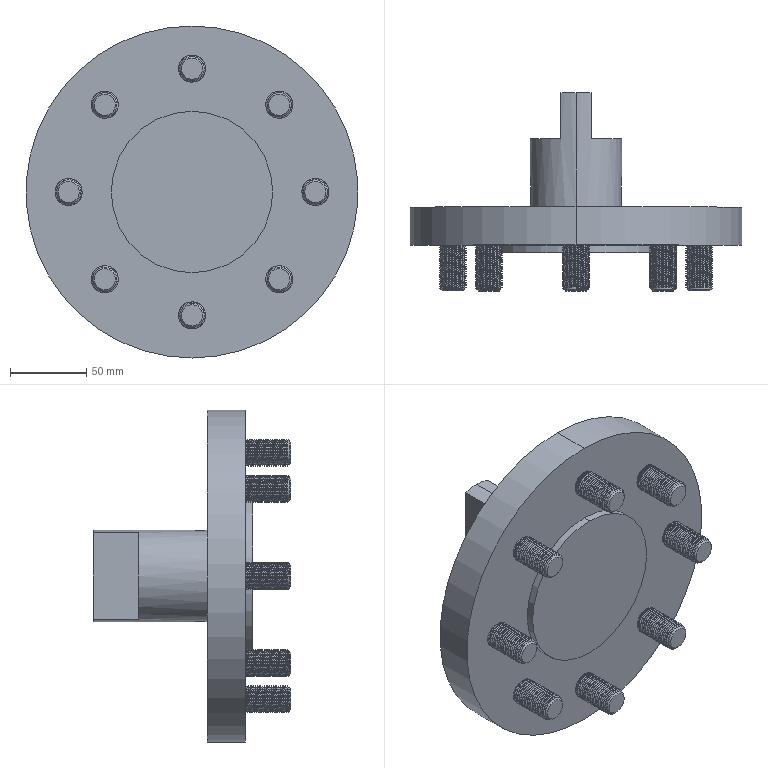Part | SolidWorks | 1 solid | 390 faces | box 218 x 130 x 218 mm | volume 1192193 mm3 | cylinder 326 | plane 24 | spline 24 | cone 16 | commonest cylinder face diameters 16 x320 60 x2 106 x2 218 x2